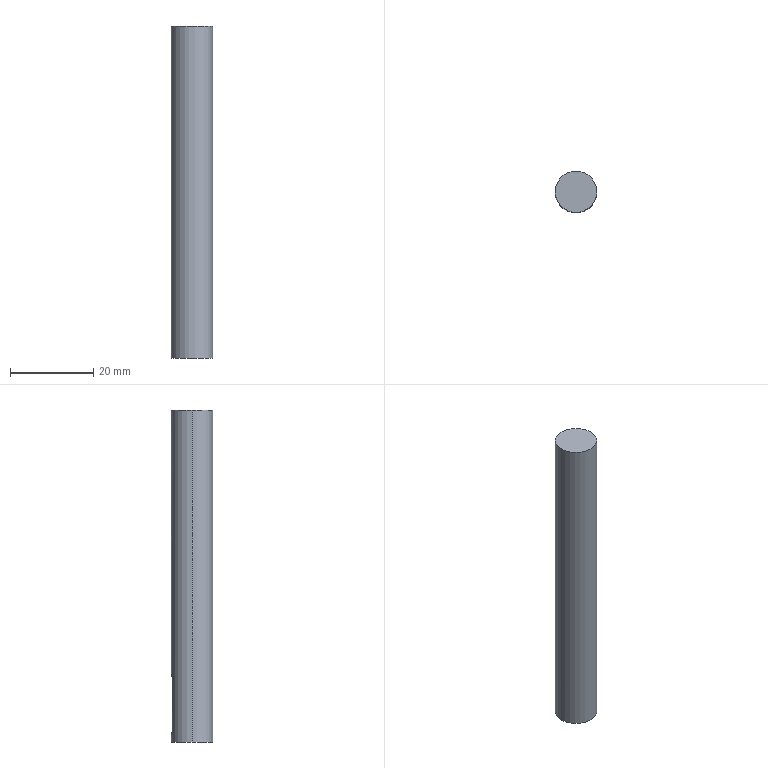Part | SolidWorks | features Extrusion 1, ICE 1 | 1 solid | 10 faces | box 10 x 10 x 80 mm | volume 6158 mm3 | cylinder 5 | plane 5 | commonest cylinder face diameters 3.039 x3 10 x2
STEP:
#1=CARTESIAN_POINT('',(0.,2.,16.52));
#2=VERTEX_POINT('',#1);
#3=CARTESIAN_POINT('',(1.52,2.,15.));
#4=VERTEX_POINT('',#3);
#5=CARTESIAN_POINT('',(0.,2.,15.));
#6=DIRECTION('',(0.,1.,0.));
#7=DIRECTION('',(0.,0.,1.));
#8=AXIS2_PLACEMENT_3D('',#5,#6,#7);
#9=CIRCLE('',#8,1.52);
#10=EDGE_CURVE('',#2,#4,#9,.T.);
#11=ORIENTED_EDGE('',*,*,#10,.F.);
#12=CARTESIAN_POINT('',(0.,5.,16.52));
#13=VERTEX_POINT('',#12);
#14=CARTESIAN_POINT('',(0.,2.,16.52));
#15=DIRECTION('',(0.,1.,0.));
#16=VECTOR('',#15,1000.);
#17=LINE('',#14,#16);
#18=EDGE_CURVE('',#2,#13,#17,.T.);
#19=ORIENTED_EDGE('',*,*,#18,.T.);
#20=CARTESIAN_POINT('',(1.52,4.763,15.));
#21=VERTEX_POINT('',#20);
#22=CARTESIAN_POINT('',(1.52,4.763,15.));
#23=CARTESIAN_POINT('',(1.52,4.763,15.101));
#24=CARTESIAN_POINT('',(1.51,4.767,15.2));
#25=CARTESIAN_POINT('',(1.471,4.779,15.395));
#26=CARTESIAN_POINT('',(1.441,4.788,15.492));
#27=CARTESIAN_POINT('',(1.365,4.81,15.676));
#28=CARTESIAN_POINT('',(1.318,4.824,15.763));
#29=CARTESIAN_POINT('',(1.207,4.852,15.928));
#30=CARTESIAN_POINT('',(1.144,4.868,16.005));
#31=CARTESIAN_POINT('',(0.9347,4.914,16.214));
#32=CARTESIAN_POINT('',(0.766,4.944,16.327));
#33=CARTESIAN_POINT('',(0.4005,4.987,16.479));
#34=CARTESIAN_POINT('',(0.1997,5.,16.52));
#35=CARTESIAN_POINT('',(0.,5.,16.52));
#36=B_SPLINE_CURVE_WITH_KNOTS('',3,(#22,#23,#24,#25,#26,#27,#28,#29,#30,#31,#32,#33,#34,#35),.UNSPECIFIED.,.F.,.F.,(4,2,2,2,2,2,4),(0.,0.0002988,0.0005976,0.0008964,0.001195,0.001793,0.00239),.UNSPECIFIED.);
#37=EDGE_CURVE('',#21,#13,#36,.T.);
#38=ORIENTED_EDGE('',*,*,#37,.F.);
#39=CARTESIAN_POINT('',(1.52,2.,15.));
#40=DIRECTION('',(0.,1.,0.));
#41=VECTOR('',#40,1000.);
#42=LINE('',#39,#41);
#43=EDGE_CURVE('',#4,#21,#42,.T.);
#44=ORIENTED_EDGE('',*,*,#43,.F.);
#45=EDGE_LOOP('',(#11,#19,#38,#44));
#46=FACE_OUTER_BOUND('',#45,.T.);
#47=CARTESIAN_POINT('',(0.,2.,15.));
#48=DIRECTION('',(0.,1.,0.));
#49=DIRECTION('',(0.,0.,1.));
#50=AXIS2_PLACEMENT_3D('',#47,#48,#49);
#51=CYLINDRICAL_SURFACE('',#50,1.52);
#52=ADVANCED_FACE('',(#46),#51,.F.);
#53=CARTESIAN_POINT('',(-1.52,4.763,15.));
#54=VERTEX_POINT('',#53);
#55=CARTESIAN_POINT('',(-1.52,4.763,3.26));
#56=VERTEX_POINT('',#55);
#57=CARTESIAN_POINT('',(-1.52,4.763,80.));
#58=DIRECTION('',(0.,0.,-1.));
#59=VECTOR('',#58,1000.);
#60=LINE('',#57,#59);
#61=EDGE_CURVE('',#54,#56,#60,.T.);
#62=ORIENTED_EDGE('',*,*,#61,.T.);
#63=CARTESIAN_POINT('',(1.52,4.763,3.26));
#64=VERTEX_POINT('',#63);
#65=CARTESIAN_POINT('',(-1.52,4.763,3.26));
#66=CARTESIAN_POINT('',(-1.52,4.763,3.159));
#67=CARTESIAN_POINT('',(-1.51,4.767,3.06));
#68=CARTESIAN_POINT('',(-1.471,4.779,2.865));
#69=CARTESIAN_POINT('',(-1.441,4.788,2.768));
#70=CARTESIAN_POINT('',(-1.365,4.81,2.584));
#71=CARTESIAN_POINT('',(-1.318,4.823,2.497));
#72=CARTESIAN_POINT('',(-1.208,4.852,2.332));
#73=CARTESIAN_POINT('',(-1.144,4.868,2.255));
#74=CARTESIAN_POINT('',(-0.9354,4.914,2.046));
#75=CARTESIAN_POINT('',(-0.7669,4.944,1.933));
#76=CARTESIAN_POINT('',(-0.4017,4.987,1.781));
#77=CARTESIAN_POINT('',(-0.201,5.,1.74));
#78=CARTESIAN_POINT('',(0.09825,5.,1.74));
#79=CARTESIAN_POINT('',(0.1996,4.997,1.75));
#80=CARTESIAN_POINT('',(0.395,4.985,1.789));
#81=CARTESIAN_POINT('',(0.49,4.977,1.818));
#82=CARTESIAN_POINT('',(0.7672,4.944,1.933));
#83=CARTESIAN_POINT('',(0.9339,4.914,2.045));
#84=CARTESIAN_POINT('',(1.144,4.868,2.255));
#85=CARTESIAN_POINT('',(1.207,4.853,2.331));
#86=CARTESIAN_POINT('',(1.317,4.824,2.495));
#87=CARTESIAN_POINT('',(1.365,4.81,2.584));
#88=CARTESIAN_POINT('',(1.479,4.777,2.858));
#89=CARTESIAN_POINT('',(1.52,4.763,3.058));
#90=CARTESIAN_POINT('',(1.52,4.763,3.26));
#91=B_SPLINE_CURVE_WITH_KNOTS('',3,(#65,#66,#67,#68,#69,#70,#71,#72,#73,#74,#75,#76,#77,#78,#79,#80,#81,#82,#83,#84,#85,#86,#87,#88,#89,#90),.UNSPECIFIED.,.F.,.F.,(4,2,2,2,2,2,2,2,2,2,2,2,4),(0.,0.0002986,0.0005972,0.0008958,0.001194,0.001792,0.002389,0.002687,0.002986,0.003583,0.003882,0.00418,0.004778),.UNSPECIFIED.);
#92=EDGE_CURVE('',#56,#64,#91,.T.);
#93=ORIENTED_EDGE('',*,*,#92,.T.);
#94=CARTESIAN_POINT('',(1.52,4.763,80.));
#95=DIRECTION('',(0.,0.,1.));
#96=VECTOR('',#95,1000.);
#97=LINE('',#94,#96);
#98=EDGE_CURVE('',#64,#21,#97,.T.);
#99=ORIENTED_EDGE('',*,*,#98,.T.);
#100=ORIENTED_EDGE('',*,*,#37,.T.);
#101=CARTESIAN_POINT('',(0.,5.,16.52));
#102=CARTESIAN_POINT('',(-0.0997,5.,16.52));
#103=CARTESIAN_POINT('',(-0.201,4.997,16.51));
#104=CARTESIAN_POINT('',(-0.3962,4.985,16.47));
#105=CARTESIAN_POINT('',(-0.4911,4.977,16.441));
#106=CARTESIAN_POINT('',(-0.768,4.944,16.326));
#107=CARTESIAN_POINT('',(-0.9346,4.914,16.214));
#108=CARTESIAN_POINT('',(-1.145,4.868,16.004));
#109=CARTESIAN_POINT('',(-1.207,4.852,15.928));
#110=CARTESIAN_POINT('',(-1.317,4.824,15.764));
#111=CARTESIAN_POINT('',(-1.365,4.81,15.675));
#112=CARTESIAN_POINT('',(-1.479,4.777,15.401));
#113=CARTESIAN_POINT('',(-1.52,4.763,15.202));
#114=CARTESIAN_POINT('',(-1.52,4.763,15.));
#115=B_SPLINE_CURVE_WITH_KNOTS('',3,(#101,#102,#103,#104,#105,#106,#107,#108,#109,#110,#111,#112,#113,#114),.UNSPECIFIED.,.F.,.F.,(4,2,2,2,2,2,4),(0.00239,0.002689,0.002987,0.003584,0.003882,0.004181,0.004778),.UNSPECIFIED.);
#116=EDGE_CURVE('',#13,#54,#115,.T.);
#117=ORIENTED_EDGE('',*,*,#116,.T.);
#118=EDGE_LOOP('',(#62,#93,#99,#100,#117));
#119=FACE_BOUND('',#118,.T.);
#120=CARTESIAN_POINT('',(5.,0.,80.));
#121=VERTEX_POINT('',#120);
#122=CARTESIAN_POINT('',(-5.,0.,80.));
#123=VERTEX_POINT('',#122);
#124=CARTESIAN_POINT('',(0.,0.,80.));
#125=DIRECTION('',(0.,0.,1.));
#126=DIRECTION('',(1.,0.,0.));
#127=AXIS2_PLACEMENT_3D('',#124,#125,#126);
#128=CIRCLE('',#127,5.);
#129=EDGE_CURVE('',#121,#123,#128,.T.);
#130=ORIENTED_EDGE('',*,*,#129,.F.);
#131=CARTESIAN_POINT('',(5.,0.,0.));
#132=VERTEX_POINT('',#131);
#133=CARTESIAN_POINT('',(5.,0.,80.));
#134=DIRECTION('',(0.,0.,-1.));
#135=VECTOR('',#134,1000.);
#136=LINE('',#133,#135);
#137=EDGE_CURVE('',#121,#132,#136,.T.);
#138=ORIENTED_EDGE('',*,*,#137,.T.);
#139=CARTESIAN_POINT('',(-5.,0.,0.));
#140=VERTEX_POINT('',#139);
#141=CARTESIAN_POINT('',(0.,0.,0.));
#142=DIRECTION('',(0.,0.,1.));
#143=DIRECTION('',(1.,0.,0.));
#144=AXIS2_PLACEMENT_3D('',#141,#142,#143);
#145=CIRCLE('',#144,5.);
#146=EDGE_CURVE('',#132,#140,#145,.T.);
#147=ORIENTED_EDGE('',*,*,#146,.T.);
#148=CARTESIAN_POINT('',(-5.,0.,80.));
#149=DIRECTION('',(0.,0.,-1.));
#150=VECTOR('',#149,1000.);
#151=LINE('',#148,#150);
#152=EDGE_CURVE('',#123,#140,#151,.T.);
#153=ORIENTED_EDGE('',*,*,#152,.F.);
#154=EDGE_LOOP('',(#130,#138,#147,#153));
#155=FACE_OUTER_BOUND('',#154,.T.);
#156=CARTESIAN_POINT('',(0.,0.,80.));
#157=DIRECTION('',(0.,0.,-1.));
#158=DIRECTION('',(-1.,0.,0.));
#159=AXIS2_PLACEMENT_3D('',#156,#157,#158);
#160=CYLINDRICAL_SURFACE('',#159,5.);
#161=ADVANCED_FACE('',(#119,#155),#160,.T.);
#162=ORIENTED_EDGE('',*,*,#137,.F.);
#163=CARTESIAN_POINT('',(0.,0.,80.));
#164=DIRECTION('',(0.,0.,1.));
#165=DIRECTION('',(1.,0.,0.));
#166=AXIS2_PLACEMENT_3D('',#163,#164,#165);
#167=CIRCLE('',#166,5.);
#168=EDGE_CURVE('',#123,#121,#167,.T.);
#169=ORIENTED_EDGE('',*,*,#168,.F.);
#170=ORIENTED_EDGE('',*,*,#152,.T.);
#171=CARTESIAN_POINT('',(0.,0.,0.));
#172=DIRECTION('',(0.,0.,1.));
#173=DIRECTION('',(1.,0.,0.));
#174=AXIS2_PLACEMENT_3D('',#171,#172,#173);
#175=CIRCLE('',#174,5.);
#176=EDGE_CURVE('',#140,#132,#175,.T.);
#177=ORIENTED_EDGE('',*,*,#176,.T.);
#178=EDGE_LOOP('',(#162,#169,#170,#177));
#179=FACE_OUTER_BOUND('',#178,.T.);
#180=CARTESIAN_POINT('',(0.,0.,80.));
#181=DIRECTION('',(0.,0.,-1.));
#182=DIRECTION('',(-1.,0.,0.));
#183=AXIS2_PLACEMENT_3D('',#180,#181,#182);
#184=CYLINDRICAL_SURFACE('',#183,5.);
#185=ADVANCED_FACE('',(#179),#184,.T.);
#186=ORIENTED_EDGE('',*,*,#168,.T.);
#187=ORIENTED_EDGE('',*,*,#129,.T.);
#188=EDGE_LOOP('',(#186,#187));
#189=FACE_OUTER_BOUND('',#188,.T.);
#190=CARTESIAN_POINT('',(0.,0.,80.));
#191=DIRECTION('',(0.,0.,1.));
#192=DIRECTION('',(1.,0.,0.));
#193=AXIS2_PLACEMENT_3D('',#190,#191,#192);
#194=PLANE('',#193);
#195=ADVANCED_FACE('',(#189),#194,.T.);
#196=ORIENTED_EDGE('',*,*,#176,.F.);
#197=ORIENTED_EDGE('',*,*,#146,.F.);
#198=EDGE_LOOP('',(#196,#197));
#199=FACE_OUTER_BOUND('',#198,.T.);
#200=CARTESIAN_POINT('',(0.,0.,0.));
#201=DIRECTION('',(0.,0.,1.));
#202=DIRECTION('',(1.,0.,0.));
#203=AXIS2_PLACEMENT_3D('',#200,#201,#202);
#204=PLANE('',#203);
#205=ADVANCED_FACE('',(#199),#204,.F.);
#206=ORIENTED_EDGE('',*,*,#18,.F.);
#207=CARTESIAN_POINT('',(-1.52,2.,15.));
#208=VERTEX_POINT('',#207);
#209=CARTESIAN_POINT('',(0.,2.,15.));
#210=DIRECTION('',(0.,1.,0.));
#211=DIRECTION('',(0.,0.,1.));
#212=AXIS2_PLACEMENT_3D('',#209,#210,#211);
#213=CIRCLE('',#212,1.52);
#214=EDGE_CURVE('',#208,#2,#213,.T.);
#215=ORIENTED_EDGE('',*,*,#214,.F.);
#216=CARTESIAN_POINT('',(-1.52,2.,15.));
#217=DIRECTION('',(0.,1.,0.));
#218=VECTOR('',#217,1000.);
#219=LINE('',#216,#218);
#220=EDGE_CURVE('',#208,#54,#219,.T.);
#221=ORIENTED_EDGE('',*,*,#220,.T.);
#222=ORIENTED_EDGE('',*,*,#116,.F.);
#223=EDGE_LOOP('',(#206,#215,#221,#222));
#224=FACE_OUTER_BOUND('',#223,.T.);
#225=CARTESIAN_POINT('',(0.,2.,15.));
#226=DIRECTION('',(0.,1.,0.));
#227=DIRECTION('',(0.,0.,1.));
#228=AXIS2_PLACEMENT_3D('',#225,#226,#227);
#229=CYLINDRICAL_SURFACE('',#228,1.52);
#230=ADVANCED_FACE('',(#224),#229,.F.);
#231=ORIENTED_EDGE('',*,*,#220,.F.);
#232=CARTESIAN_POINT('',(-1.52,2.,3.26));
#233=VERTEX_POINT('',#232);
#234=CARTESIAN_POINT('',(-1.52,2.,15.));
#235=DIRECTION('',(0.,0.,1.));
#236=VECTOR('',#235,1000.);
#237=LINE('',#234,#236);
#238=EDGE_CURVE('',#233,#208,#237,.T.);
#239=ORIENTED_EDGE('',*,*,#238,.F.);
#240=CARTESIAN_POINT('',(-1.52,2.,3.26));
#241=DIRECTION('',(0.,1.,0.));
#242=VECTOR('',#241,1000.);
#243=LINE('',#240,#242);
#244=EDGE_CURVE('',#233,#56,#243,.T.);
#245=ORIENTED_EDGE('',*,*,#244,.T.);
#246=ORIENTED_EDGE('',*,*,#61,.F.);
#247=EDGE_LOOP('',(#231,#239,#245,#246));
#248=FACE_OUTER_BOUND('',#247,.T.);
#249=CARTESIAN_POINT('',(-1.52,2.,15.));
#250=DIRECTION('',(-1.,0.,0.));
#251=DIRECTION('',(0.,0.,1.));
#252=AXIS2_PLACEMENT_3D('',#249,#250,#251);
#253=PLANE('',#252);
#254=ADVANCED_FACE('',(#248),#253,.F.);
#255=ORIENTED_EDGE('',*,*,#244,.F.);
#256=CARTESIAN_POINT('',(1.52,2.,3.26));
#257=VERTEX_POINT('',#256);
#258=CARTESIAN_POINT('',(0.,2.,3.26));
#259=DIRECTION('',(0.,1.,0.));
#260=DIRECTION('',(0.,0.,1.));
#261=AXIS2_PLACEMENT_3D('',#258,#259,#260);
#262=CIRCLE('',#261,1.52);
#263=EDGE_CURVE('',#257,#233,#262,.T.);
#264=ORIENTED_EDGE('',*,*,#263,.F.);
#265=CARTESIAN_POINT('',(1.52,2.,3.26));
#266=DIRECTION('',(0.,1.,0.));
#267=VECTOR('',#266,1000.);
#268=LINE('',#265,#267);
#269=EDGE_CURVE('',#257,#64,#268,.T.);
#270=ORIENTED_EDGE('',*,*,#269,.T.);
#271=ORIENTED_EDGE('',*,*,#92,.F.);
#272=EDGE_LOOP('',(#255,#264,#270,#271));
#273=FACE_OUTER_BOUND('',#272,.T.);
#274=CARTESIAN_POINT('',(0.,2.,3.26));
#275=DIRECTION('',(0.,1.,0.));
#276=DIRECTION('',(0.,0.,1.));
#277=AXIS2_PLACEMENT_3D('',#274,#275,#276);
#278=CYLINDRICAL_SURFACE('',#277,1.52);
#279=ADVANCED_FACE('',(#273),#278,.F.);
#280=ORIENTED_EDGE('',*,*,#269,.F.);
#281=CARTESIAN_POINT('',(1.52,2.,15.));
#282=DIRECTION('',(0.,0.,-1.));
#283=VECTOR('',#282,1000.);
#284=LINE('',#281,#283);
#285=EDGE_CURVE('',#4,#257,#284,.T.);
#286=ORIENTED_EDGE('',*,*,#285,.F.);
#287=ORIENTED_EDGE('',*,*,#43,.T.);
#288=ORIENTED_EDGE('',*,*,#98,.F.);
#289=EDGE_LOOP('',(#280,#286,#287,#288));
#290=FACE_OUTER_BOUND('',#289,.T.);
#291=CARTESIAN_POINT('',(1.52,2.,15.));
#292=DIRECTION('',(1.,0.,0.));
#293=DIRECTION('',(0.,0.,-1.));
#294=AXIS2_PLACEMENT_3D('',#291,#292,#293);
#295=PLANE('',#294);
#296=ADVANCED_FACE('',(#290),#295,.F.);
#297=ORIENTED_EDGE('',*,*,#214,.T.);
#298=ORIENTED_EDGE('',*,*,#10,.T.);
#299=ORIENTED_EDGE('',*,*,#285,.T.);
#300=ORIENTED_EDGE('',*,*,#263,.T.);
#301=ORIENTED_EDGE('',*,*,#238,.T.);
#302=EDGE_LOOP('',(#297,#298,#299,#300,#301));
#303=FACE_OUTER_BOUND('',#302,.T.);
#304=CARTESIAN_POINT('',(0.,2.,15.));
#305=DIRECTION('',(0.,1.,0.));
#306=DIRECTION('',(0.,0.,1.));
#307=AXIS2_PLACEMENT_3D('',#304,#305,#306);
#308=PLANE('',#307);
#309=ADVANCED_FACE('',(#303),#308,.T.);
#310=CLOSED_SHELL('',(#52,#161,#185,#195,#205,#230,#254,#279,#296,#309));
#311=MANIFOLD_SOLID_BREP('',#310);
#312=CARTESIAN_POINT('',(0.,0.,0.));
#313=DIRECTION('',(0.,0.,1.));
#314=DIRECTION('',(1.,0.,0.));
#315=AXIS2_PLACEMENT_3D('',#312,#313,#314);
#316=(LENGTH_UNIT()NAMED_UNIT(*)SI_UNIT(.MILLI.,.METRE.));
#317=UNCERTAINTY_MEASURE_WITH_UNIT(LENGTH_MEASURE(0.00001),#316,'','');
#318=(NAMED_UNIT(*)PLANE_ANGLE_UNIT()SI_UNIT($,.RADIAN.));
#319=(NAMED_UNIT(*)SI_UNIT($,.STERADIAN.)SOLID_ANGLE_UNIT());
#320=(GEOMETRIC_REPRESENTATION_CONTEXT(3)GLOBAL_UNCERTAINTY_ASSIGNED_CONTEXT((#317))GLOBAL_UNIT_ASSIGNED_CONTEXT((#316,#318,#319))REPRESENTATION_CONTEXT('',''));
#321=ADVANCED_BREP_SHAPE_REPRESENTATION('',(#311,#315),#320);